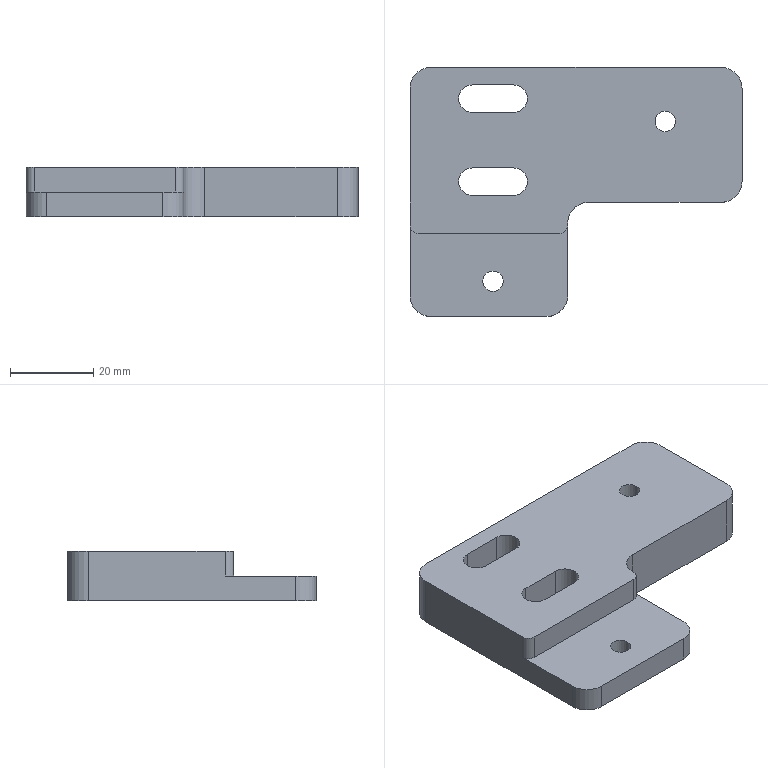NC program | NX | posted with a generic post | part box 80 x 60 x 12 mm
Lines 19 to 945 of 5338:
(ADAPTIVE_MILLING , TOOL : D10)
N36 T15 M6
N38 G54
N40 G17 G0 G90 X-52.678 Y3.969 S9500 M3
N42 G43 Z30. H15
N44 Z-9.
N46 G94 G1 Z-12. F1000.
N48 X-51.955 Y3.649 F3500.
N50 X-51.222 Y3.352
N52 G3 X-50.031 Y3.969 R1.015
N54 X-49.59 Y7.203 R11.435
N56 X-49.506 Y16.827 R445.113
N58 G2 X-49.477 Y33.326 R953.284
N60 X-46.244 Y37.824 R6.109
N62 X-40.67 Y39.298 R13.456
N64 X-30.424 Y39.492 R151.23
N66 G1 X-24.674 Y39.494
N68 X42.826
N70 X42.951 Y39.492
N72 X43.076 Y39.487
N74 X43.138 Y39.483
N76 X43.263 Y39.472
N78 G2 X47.822 Y36.232 R6.088
N80 X49.287 Y30.783 R13.246
N82 X49.492 Y20.413 R143.675
N84 G1 X49.494 Y14.85
N86 Y-32.837
N88 X49.492 Y-32.962
N90 X49.487 Y-33.087
N92 X49.483 Y-33.15
N94 X49.472 Y-33.274
N96 G2 X46.278 Y-37.797 R6.078
N98 X40.71 Y-39.294 R13.263
N100 X31.027 Y-39.491 R137.718
N102 G1 X26.59 Y-39.493
N104 X-35.848 Y-39.494
N106 X-36.098 Y-39.495
N108 X-42.848
N110 X-42.973 Y-39.492
N112 X-43.098 Y-39.487
N114 G2 X-47.739 Y-36.377 R5.989
N116 X-49.266 Y-31.012 R12.765
N118 X-49.491 Y-21.58 R116.088
N120 G1 X-49.494 Y-17.955
N122 Y1.295
N124 X-49.491 Y1.545
N126 X-49.483 Y1.795
N128 X-49.473 Y2.045
N130 G3 X-49.015 Y15.406 R138.865
N132 G2 X-48.982 Y31.281 R941.095
N134 X-44.875 Y37.18 R7.48
N136 X-38.995 Y38.738 R15.237
N138 X-29.501 Y38.983 R119.88
N140 G1 X-26.813 Y38.987
N142 X-20.001 Y38.988
N144 X40.687
N146 X40.812 Y38.986
N148 X40.937 Y38.983
N150 X41.124 Y38.973
N152 G2 X47.135 Y34.939 R7.429
N154 X48.754 Y28.822 R15.356
N156 X48.985 Y18.827 R132.025
N158 G1 X48.988 Y15.452
N160 X48.989 Y-0.298
N162 Y-30.673
N164 X48.987 Y-30.798
N166 X48.981 Y-30.985
N168 X48.975 Y-31.11
N170 G2 X44.898 Y-37.158 R7.437
N172 X38.899 Y-38.747 R15.354
N174 X28.53 Y-38.985 R135.396
N176 G1 X24.842 Y-38.988
N178 X-3.845
N180 X-33.72 Y-38.989
N182 X-35.845
N184 X-40.658
N186 X-40.783 Y-38.988
N188 G2 X-47.121 Y-34.966 R7.396
N190 X-48.734 Y-29.039 R15.01
N192 X-48.982 Y-20.17 R108.447
N194 G1 X-48.986 Y-17.92
N196 X-48.988 Y-13.482
N198 Y-0.42
N200 X-48.985 Y0.08
N202 X-48.979 Y0.392
N204 X-48.968 Y0.83
N206 G3 X-48.519 Y18.07 R239.849
N208 G2 X-48.482 Y29.632 R716.485
N210 X-43.532 Y36.705 R8.46
N212 X-37.316 Y38.227 R17.447
N214 X-27.509 Y38.477 R128.145
N216 G1 X-24.822 Y38.481
N218 X-18.884 Y38.483
N220 X23.928
N222 X24.241 Y38.484
N224 X24.803
N226 X25.116 Y38.485
N228 G2 X39.678 Y38.452 R836.944
N230 X46.698 Y33.525 R8.442
N232 X48.256 Y26.999 R17.862
N234 X48.481 Y15.129 R177.604
N236 G1 X48.483 Y9.879
N238 Y-28.746
N240 X48.481 Y-28.996
N242 X48.477 Y-29.184
N244 X48.473 Y-29.309
N246 X48.464 Y-29.496
N248 G2 X43.52 Y-36.701 R8.44
N250 X36.993 Y-38.255 R17.932
N252 X26.123 Y-38.479 R161.092
N254 G1 X22.373 Y-38.482
N256 X-1.002 Y-38.483
N258 X-23.377
N260 X-23.689 Y-38.484
N262 X-24.252
N264 X-24.564 Y-38.485
N266 G2 X-39.689 Y-38.454 R869.538
N268 X-46.704 Y-33.517 R8.449
N270 X-48.245 Y-27.115 R17.733
N272 X-48.48 Y-15.995 R158.486
N274 X-48.427 Y1.004 R748.676
N276 G3 X-48.025 Y18.685 R293.67
N278 G2 X-47.965 Y28.433 R262.553
N280 X-42.389 Y36.207 R9.207
N282 X-35.598 Y37.743 R19.721
N284 X-23.165 Y37.975 R191.105
N286 G1 X-18.165 Y37.977
N288 X21.835 Y37.978
N290 X22.273 Y37.979
N292 X22.71 Y37.98
N294 X23.148 Y37.981
N296 X24.585 Y37.98
N298 G2 X38.334 Y37.943 R554.072
N300 X46.194 Y32.397 R9.198
N302 X47.727 Y25.797 R19.223
N304 X47.973 Y15.115 R152.13
N306 G1 X47.976 Y12.177
N308 X47.978 Y4.927
N310 Y-27.073
N312 X47.976 Y-27.385
N314 X47.971 Y-27.635
N316 X47.968 Y-27.76
N318 G2 X42.406 Y-36.188 R9.21
N320 X35.557 Y-37.743 R19.566
N322 X23.749 Y-37.974 R179.522
N324 G1 X19.437 Y-37.977
N326 X-21.251 Y-37.978
N328 X-22.376 Y-37.979
N330 X-22.813 Y-37.98
N332 X-24.626
N334 X-26.063 Y-37.981
N336 G2 X-38.313 Y-37.944 R530.442
N338 X-46.185 Y-32.418 R9.187
N340 X-47.724 Y-25.819 R19.251
N342 X-47.974 Y-14.324 R163.209
N344 X-47.899 Y1.05 R522.369
N346 G3 X-47.526 Y22.169 R410.142
N348 G2 X-47.395 Y27.851 R55.442
N350 X-41.366 Y35.698 R9.806
N352 X-34.567 Y37.213 R20.757
N354 X-23.635 Y37.466 R154.256
N356 G1 X-20.76 Y37.47
N358 X-14.385 Y37.472
N360 X19.553
N362 X20.115 Y37.474
N364 X20.678
N366 X21.178 Y37.476
N368 G2 X36.865 Y37.45 R878.1
N370 X45.705 Y31.332 R9.835
N372 X47.23 Y24.345 R21.115
N374 X47.469 Y11.912 R192.215
N376 G1 X47.472 Y7.474
N378 Y-25.588
N380 X47.47 Y-25.901
N382 X47.464 Y-26.275
N384 X47.457 Y-26.525
N386 X47.447 Y-26.775
N388 G2 X41.351 Y-35.693 R9.827
N390 X34.366 Y-37.227 R21.025
N392 X22.058 Y-37.469 R187.16
N394 G1 X17.621 Y-37.472
N396 X-19.067
N398 X-19.567 Y-37.474
N400 X-20.379
N402 X-21.067 Y-37.475
N404 X-22.442
N406 G2 X-36.941 Y-37.445 R794.612
N408 X-45.735 Y-31.262 R9.832
N410 X-47.246 Y-24.144 R21.676
N412 X-47.468 Y-12.961 R184.381
N414 X-47.154 Y7.847 R395.574
N416 G3 X-47.008 Y25.033 R897.934
N418 G2 X-45.105 Y31.525 R11.201
N420 X-38.676 Y35.814 R11.777
N422 X-31.077 Y36.842 R31.833
N424 X-12.078 Y36.967 R673.573
N426 G1 X17.422
N428 X19.922 Y36.97
N430 X21.422 Y36.971
N432 X21.859 Y36.973
N434 X22.546 Y36.974
N436 X23.359
N438 G2 X35.796 Y36.94 R601.467
N440 X45.211 Y30.341 R10.368
N442 X46.723 Y23.157 R22.585
N444 X46.964 Y10.099 R209.815
N446 G1 X46.967 Y5.287
N448 Y-24.213
N450 X46.963 Y-24.713
N452 X46.958 Y-25.026
N454 X46.95 Y-25.338
N456 G2 X44.37 Y-32.399 R10.607
N458 X37.985 Y-35.996 R12.565
N460 X30.049 Y-36.876 R37.4
N462 X13.987 Y-36.966 R769.024
N464 G1 X-16.888 Y-36.967
N466 X-17.325 Y-36.968
N468 X-18.263 Y-36.969
N470 X-19.513 Y-36.97
N472 X-20.263
N474 X-20.763 Y-36.971
N476 G2 X-35.824 Y-36.936 R721.83
N478 X-45.174 Y-30.43 R10.334
N480 X-46.712 Y-23.316 R22.255
N482 X-46.963 Y-11.383 R181.717
N484 X-46.662 Y7.862 R420.02
N486 G3 X-46.505 Y24.049 R969.988
N488 G2 X-44.748 Y30.472 R12.025
N490 X-38.349 Y35.114 R11.8
N492 X-30.526 Y36.307 R29.809
N494 X-13.59 Y36.461 R466.972
N496 G1 X15.223 Y36.462
N498 X16.035
N500 X16.473 Y36.464
N502 X16.91
N504 X17.223 Y36.465
N506 X18.535
N508 G2 X34.597 Y36.44 R831.129
N510 X41.935 Y33.566 R11.003
N512 X45.507 Y26.949 R13.263
N514 X46.376 Y18.635 R40.48
N516 X46.462 Y0.51 R850.421
N518 G1 Y-22.865
N520 X46.458 Y-23.427
N522 X46.453 Y-23.74
N524 X46.444 Y-24.114
N526 X46.436 Y-24.364
N528 G2 X44.121 Y-31.289 R11.301
N530 X37.648 Y-35.319 R12.461
N532 X29.858 Y-36.334 R33.754
N534 X12.296 Y-36.461 R612.464
N536 G1 X-14.704 Y-36.462
N538 X-15.141 Y-36.463
N540 X-16.141 Y-36.464
N542 X-16.641 Y-36.465
N544 X-18.078
N546 X-18.516 Y-36.466
N548 G2 X-34.765 Y-36.428 R731.931
N550 X-44.669 Y-29.518 R10.799
N552 X-46.194 Y-22.335 R23.117
N554 X-46.457 Y-10.153 R180.72
N556 X-46.151 Y8.531 R482.227
N558 G3 X-46.014 Y22.718 R881.104
N560 G2 X-44.715 Y28.837 R13.812
N562 X-42.3 Y31.949 R10.683
N564 X-38.4 Y34.48 R10.149
N566 X-31.457 Y35.691 R27.998
N568 X-19.337 Y35.95 R192.668
N570 G1 X-16.275 Y35.954
N572 X-10.087 Y35.956
N574 X13.038
N576 X13.913 Y35.957
N578 X14.35 Y35.959
N580 X14.913
N582 X15.788 Y35.96
N584 X16.1 Y35.961
N586 X16.6
N588 X16.913 Y35.963
N590 X17.475
N592 X17.85 Y35.964
N594 X18.163
N596 X18.538 Y35.966
N598 X19.038
N600 X19.975 Y35.97
N602 X20.538 Y35.969
N604 X21.913 Y35.973
N606 X22.85 Y35.976
N608 X23.35
N610 X23.725 Y35.977
N612 X25.288 Y35.975
N614 X26.163 Y35.978
N616 X26.663 Y35.977
N618 X27.288 Y35.979
N620 X27.663
N622 X28.413 Y35.981
N624 X28.913 Y35.98
N626 X29.35 Y35.981
N628 G2 X35.217 Y35.785 R46.802
N630 X41.859 Y32.374 R10.751
N632 G1 X42.103 Y32.174
N634 X42.174 Y32.103
N636 X43.366 Y30.65
N638 X43.422 Y30.567
N640 G2 X44.442 Y28.519 R12.875
N642 X45.67 Y21.706 R27.357
N644 X45.952 Y8.337 R197.475
N646 G1 X45.955 Y4.587
N648 X45.956 Y-6.163
N650 Y-21.663
N652 X45.952 Y-22.226
N654 X45.945 Y-22.726
N656 X45.936 Y-23.101
N658 G2 X44.27 Y-29.558 R12.646
N660 X37.727 Y-34.507 R11.976
N662 X30.041 Y-35.766 R28.902
N664 X14.044 Y-35.955 R359.108
N666 G1 X-0.956 Y-35.956
N668 X-12.519
N670 X-13.019 Y-35.958
N672 X-14.019 Y-35.959
N674 X-14.456 Y-35.96
N676 X-15.644
N678 G2 X-33.643 Y-35.926 R895.197
N680 X-40.761 Y-33.419 R11.64
N682 X-43.422 Y-30.567 R16.586
N684 X-44.442 Y-28.519 R12.875
N686 X-45.681 Y-21.581 R27.69
N688 X-45.949 Y-9.837 R179.438
N690 X-45.644 Y9.347 R619.345
N692 G1 X-45.614 Y11.034
N694 X-45.597 Y12.097
N696 X-45.584 Y13.534
N698 X-45.572 Y15.221
N700 X-45.566 Y16.409
N702 X-45.563 Y16.846
N704 X-45.561 Y17.346
N706 X-45.558 Y17.784
N708 X-45.556 Y18.159
N710 X-45.548 Y19.159
N712 X-45.547 Y19.471
N714 X-45.537 Y20.409
N716 X-45.526 Y21.221
N718 X-45.516 Y21.659
N720 X-45.503 Y22.096
N722 X-45.49 Y22.408
N724 G2 X-45.012 Y25.891 R17.523
N726 G1 X-44.911 Y26.92
N728 X-44.891 Y27.019
N730 X-44.346 Y28.817
N732 X-44.307 Y28.91
N734 X-43.422 Y30.567
N736 X-43.366 Y30.65
N738 X-42.295 Y31.955
N740 X-42.103 Y32.174
N742 X-41.341 Y32.806
N744 X-40.567 Y33.422
N746 X-39.697 Y33.893
N748 X-38.817 Y34.346
N750 X-37.019 Y34.891
N752 G2 X-32.663 Y35.155 R39.026
N754 X-16.23 Y35.447 R314.936
N756 G1 X-11.418 Y35.45
N758 X10.895 Y35.451
N760 X11.77 Y35.452
N762 X12.27 Y35.454
N764 X12.832
N766 X13.707 Y35.455
N768 X14.145 Y35.457
N770 X14.707
N772 X15.457 Y35.458
N774 X15.895 Y35.46
N776 X16.332
N778 X17.082 Y35.461
N780 X18.27 Y35.464
N782 X18.582
N784 X19.02 Y35.466
N786 X20.395 Y35.468
N788 X21.332 Y35.47
N790 X22.207 Y35.471
N792 X23.207
N794 X23.707 Y35.472
N796 X24.332 Y35.473
N798 X24.582
N800 X25.02 Y35.474
N802 X26.02 Y35.475
N804 X27.707 Y35.476
N806 G2 X34.138 Y35.299 R59.033
N808 G3 X37.019 Y34.891 R34.04
N810 G1 X38.817 Y34.346
N812 X38.91 Y34.307
N814 X40.567 Y33.422
N816 X40.65 Y33.366
N818 X41.907 Y32.335
N820 G3 X43.412 Y32.617 R1.003
N822 X43.466 Y33.5 Z-11.954 R1.05
N824 G1 X43.142 Y34.537 Z-11.9
N826 X42.635 Y36.159
N828 G3 X41.907 Y36.835 R1.014
N830 G1 X38.497 Y37.613
N832 G3 X30.566 Y38.446 R43.677
N834 G1 X29.568 Y38.454
N836 X-29.332 Y38.314
N838 X-30.98 Y38.282
N840 X-31.144 Y38.26
N842 X-31.304 Y38.22
N844 X-32.966 Y37.607
N846 X-34.617 Y36.991 Z-11.988
N848 X-34.814 Y36.858 Z-12.
N850 G3 X-34.162 Y35.1 R1.001
N852 G1 X34.975
N854 X35.025 Y35.098
N856 X35.647 Y35.036
N858 X36.334 Y34.972
N860 X37.019 Y34.891
N862 X37.968 Y34.61
N864 X38.91 Y34.307
N866 X39.785 Y33.846
N868 X40.65 Y33.366
N870 X41.419 Y32.742
N872 X42.174 Y32.103
N874 X42.806 Y31.341
N876 X43.422 Y30.567
N878 X43.893 Y29.697
N880 X44.346 Y28.817
N882 X44.891 Y27.019
N884 G2 X45.137 Y23.038 R31.355
N886 X45.449 Y4.73 R341.606
N888 G1 X45.451 Y-2.707
N890 Y-20.52
N892 X45.446 Y-21.145
N894 X45.441 Y-21.582
N896 X45.431 Y-22.019
N898 G2 X44.027 Y-28.303 R13.841
N900 X37.349 Y-33.834 R11.954
N902 X29.375 Y-35.239 R28.194
N904 X15.816 Y-35.448 R271.557
N906 G1 X10.754 Y-35.45
N908 X-10.246 Y-35.451
N910 X-10.809 Y-35.453
N912 X-11.871
N914 X-12.309 Y-35.455
N916 X-13.559
N918 X-13.996 Y-35.457
N920 X-14.621
N922 X-15.059 Y-35.459
N924 X-15.434
N926 X-15.809 Y-35.461
N928 X-18.121 Y-35.462
N930 X-18.434 Y-35.464
N932 X-19.246
N934 X-19.809 Y-35.466
N936 X-20.559
N938 X-20.996 Y-35.467
N940 X-21.434
N942 X-21.996 Y-35.469
N944 X-24.246 Y-35.468
N946 X-25.121 Y-35.469
N948 X-25.559 Y-35.47
N950 X-27.559
N952 G2 X-34.115 Y-35.298 R62.042
N954 G3 X-37.019 Y-34.891 R35.555
N956 G1 X-38.817 Y-34.346
N958 X-38.91 Y-34.307
N960 X-40.567 Y-33.422
N962 X-40.65 Y-33.366
N964 X-41.858 Y-32.374
N966 G3 X-43.408 Y-32.714 R1.013
N968 G1 X-43.716 Y-33.336
N970 X-43.999 Y-33.968
N972 G3 X-42.476 Y-35.092 R1.011
N974 G1 Z-9.
N976 G0 Z53.
N978 X47.598 Y23.655
N980 Z-9.
N982 G1 Z-12. F1000.
N984 G3 X46.702 Y25.451 R1.01 F3500.
N986 G1 X46.161 Y25.257
N988 X45.625 Y25.048
N990 G3 X45.1 Y24.162 R1.021
N992 G1 Y2.525
N994 X45.098 Y2.475
N996 X45.085 Y2.288
N998 G3 X44.958 Y-7.648 R217.132
N1000 G2 X44.896 Y-21.834 R589.05
N1002 X42.728 Y-28.839 R12.853
N1004 X35.905 Y-33.542 R12.934
N1006 X27.644 Y-34.774 R32.85
N1008 X11.897 Y-34.944 R414.031
N1010 G1 X1.147 Y-34.945
N1012 X-5.416
N1014 X-5.435 Y-34.946
N1016 X-6.975 Y-35.098
N1018 X-7.025 Y-35.1
N1020 X-34.975
N1022 X-35.025 Y-35.098
N1024 X-35.647 Y-35.036
N1026 G3 X-36.243 Y-36.899 R1.
N1028 G1 X-35.582 Y-37.161 Z-11.964
N1030 X-34.911 Y-37.397 Z-11.929
N1032 X-34.369 Y-37.593 Z-11.9
N1034 X-32.805 Y-38.159
N1036 X-32.637 Y-38.199
N1038 X-32.465 Y-38.218
N1040 X23.16
N1042 G3 X31.85 Y-37.499 R53.484
N1044 G1 X33.699 Y-37.193
N1046 X35.545 Y-36.87
N1048 G3 X39.608 Y-35.33 R13.765
N1050 G1 X41.159 Y-34.433
N1052 X42.699 Y-33.516
N1054 G3 X44.937 Y-31.231 R7.798
N1056 X47.702 Y-23.575 R18.416
N1058 X47.923 Y-20.596 R27.932
N1060 G1 X48.28 Y-0.707
N1062 X48.26 Y-0.515
N1064 X48.212 Y-0.328
N1066 X47.523 Y1.451
N1068 X47.251 Y2.168 Z-11.938
N1070 X46.958 Y2.878 Z-11.977
N1072 X46.817 Y3.061 Z-11.988
N1074 X46.642 Y3.213 Z-12.
N1076 G3 X45.098 Y2.475 R1.002
N1078 G2 X44.671 Y-0.875 R42.456
N1080 G3 X44.468 Y-8.307 R92.385
N1082 G2 X44.375 Y-21.243 R367.805
N1084 X42.069 Y-28.332 R13.004
N1086 X34.975 Y-33.075 R13.335
N1088 X26.707 Y-34.267 R34.294
N1090 X11.896 Y-34.438 R394.662
N1092 G1 X4.709 Y-34.44
N1094 X-3.291
N1096 X-3.354
N1098 X-3.416 Y-34.443
N1100 X-3.479 Y-34.449
N1102 X-3.54 Y-34.459
N1104 X-3.561 Y-34.46
N1106 G2 X-5.453 Y-34.948 R8.588
N1108 G3 X-6.25 Y-36.389 R1.002
N1110 X-5.534 Y-36.946 Z-11.953 R1.152
N1112 G1 X-4.54 Y-37.328 Z-11.9
N1114 X-2.514 Y-38.1
N1116 X-2.271 Y-38.13
N1118 X16.479
N1120 G3 X28.916 Y-37.246 R88.684
N1122 G1 X33.862 Y-36.528
N1124 G3 X38.571 Y-34.974 R16.748
N1126 G1 X39.382 Y-34.514
N1128 X40.164 Y-34.007
N1130 X42.71 Y-32.209
N1132 G3 X43.858 Y-31.165 R6.533
N1134 G1 X44.638 Y-30.074
N1136 X45.399 Y-28.969
N1138 G3 X46.659 Y-26.003 R10.818
N1140 G1 X46.864 Y-25.092
N1142 X47.023 Y-24.172
N1144 G3 X47.4 Y-20.454 R30.837
N1146 G1 X48.073 Y-2.701
N1148 X48.053 Y-2.481
N1150 X47.993 Y-2.268
N1152 X47.227 Y-0.485
N1154 X46.969 Y0.129 Z-11.933
N1156 X46.689 Y0.733 Z-11.967
N1158 G3 X46.172 Y1.137 Z-12. R1.04
N1160 X44.891 Y0.481 R1.004
N1162 X44.059 Y-4.805 R16.614
N1164 X43.927 Y-19.054 R945.857
N1166 G2 X42.801 Y-25.414 R17.122
N1168 X35.689 Y-32.053 R12.395
N1170 X27.565 Y-33.657 R27.487
N1172 X14.946 Y-33.927 R202.133
N1174 G1 X11.946 Y-33.931
N1176 X6.571 Y-33.934
N1178 X-1.117 Y-33.935
N1180 X-1.617 Y-33.938
N1182 X-1.867 Y-33.942
N1184 X-2.054 Y-33.948
N1186 G3 X-3.183 Y-34.346 R2.382
N1188 G1 X-3.602 Y-34.473
N1190 G3 X-4.272 Y-35.709 R1.005
N1192 X-3.531 Y-36.423 Z-11.946 R1.111
N1194 G1 X-2.677 Y-36.785 Z-11.9
N1196 X-0.684 Y-37.619
N1198 X-0.42 Y-37.655
N1200 X16.455
N1202 G3 X27.648 Y-36.859 R79.831
N1204 G1 X31.563 Y-36.288
N1206 G3 X36.264 Y-35.046 R28.073
N1208 X40.025 Y-33.091 R17.846
N1210 G1 X42.078 Y-31.672
N1212 G3 X43.232 Y-30.634 R6.485
N1214 G1 X44.018 Y-29.548
N1216 X44.786 Y-28.448
N1218 G3 X46.067 Y-25.491 R10.891
N1220 G1 X46.281 Y-24.581
N1222 X46.448 Y-23.663
N1224 G3 X46.87 Y-19.949 R32.118
N1226 G1 X47.71 Y-3.897
N1228 X47.692 Y-3.669
N1230 X47.63 Y-3.448
N1232 X46.866 Y-1.679
N1234 X46.606 Y-1.066 Z-11.933
N1236 X46.325 Y-0.462 Z-11.967
N1238 G3 X45.808 Y-0.059 Z-12. R1.04
N1240 X44.528 Y-0.715 R1.004
N1242 X43.846 Y-3.157 R15.616
N1244 X43.496 Y-10.143 R54.908
N1246 G2 X43.331 Y-20.077 R185.707
N1248 X40.455 Y-27.728 R13.17
N1250 X33.132 Y-32.149 R14.342
N1252 X24.412 Y-33.278 R38.601
N1254 X8.851 Y-33.427 R508.578
N1256 G3 X-1.335 Y-33.484 R275.552
N1258 X-2.618 Y-34.055 R3.84
N1260 X-3.12 Y-35.165 R1.007
N1262 X-2.413 Y-35.918 Z-11.946 R1.108
N1264 G1 X-1.581 Y-36.317 Z-11.9
N1266 X-0.66 Y-36.765
N1268 X0.27 Y-37.193
N1270 X0.564 Y-37.237
N1272 X13.689
N1274 G3 X27.37 Y-36.265 R97.54
N1276 G1 X30.153 Y-35.872
N1278 X32.933 Y-35.457
N1280 G3 X37.927 Y-33.604 R16.39
N1282 G1 X38.569 Y-33.221
N1284 X39.199 Y-32.819
N1286 X40.969 Y-31.609
N1288 G3 X42.397 Y-30.245 R9.113
N1290 X44.176 Y-27.844 R25.524
N1292 X45.244 Y-25.469 R11.428
N1294 X46.166 Y-21.226 R17.742
N1296 G1 X46.426 Y-18.742
N1298 X46.639 Y-16.254
N1300 X47.489 Y-4.592
N1302 G3 X47.389 Y-4.076 R1.064
N1304 G1 X46.591 Y-2.462
N1306 X46.305 Y-1.871 Z-11.933
N1308 X45.997 Y-1.292 Z-11.966
N1310 G3 X45.44 Y-0.913 Z-12. R1.039
N1312 X44.307 Y-1.41 R1.007
N1314 X43.273 Y-5.045 R8.478
N1316 X42.975 Y-14.6 R110.984
N1318 G2 X42.583 Y-21.205 R41.356
N1320 X34.846 Y-30.789 R12.558
N1322 X26.889 Y-32.566 R25.976
N1324 X15.335 Y-32.908 R150.656
N1326 G3 X-0.164 Y-32.976 R823.63
N1328 X-1.433 Y-33.422 R1.799
N1330 G1 X-1.764 Y-33.598
N1332 G3 X-2.268 Y-34.703 R1.007
N1334 X-1.56 Y-35.461 Z-11.946 R1.106
N1336 G1 X-0.733 Y-35.858 Z-11.9
N1338 X0.191 Y-36.307
N1340 X1.124 Y-36.736
N1342 X1.418 Y-36.78
N1344 X6.104 Y-36.786
N1346 X10.791 Y-36.768
N1348 G3 X23.872 Y-35.952 R137.075
N1350 G1 X29.666 Y-35.297
N1352 G3 X35.088 Y-34.021 R28.468
N1354 X39.35 Y-31.863 R18.807
N1356 X42.089 Y-29.371 R14.73
N1358 G1 X43.211 Y-28.032
N1360 G3 X45.058 Y-23.989 R10.649
N1362 X45.72 Y-19.688 R23.394
N1364 X46.263 Y-5.858 R425.517
N1366 G1 X46.149 Y-4.697
N1368 X46.02 Y-3.537
N1370 X45.95 Y-2.853 Z-11.934
N1372 X45.86 Y-2.171 Z-11.969
N1374 G3 X45.525 Y-1.656 Z-12. R1.045
N1376 X44.013 Y-1.961 R1.003
N1378 X42.805 Y-5.996 R9.156
N1380 X42.48 Y-14.549 R100.058
N1382 G2 X41.984 Y-20.957 R34.687
N1384 X34.161 Y-30.277 R12.756
N1386 X26.077 Y-32.06 R26.564
N1388 X14.148 Y-32.403 R157.798
N1390 G3 X0.774 Y-32.481 R593.839
N1392 X-0.638 Y-32.781 R3.263
N1394 G1 X-1.169 Y-33.218
N1396 G3 X-1.398 Y-34.494 R1.006
N1398 X-0.497 Y-35.007 Z-11.946 R1.107
N1400 G1 X0.411 Y-35.139 Z-11.9
N1402 X1.568 Y-35.314
N1404 X2.728 Y-35.468
N1406 X20.228
N1408 G3 X28.933 Y-34.795 R59.876
N1410 X35.524 Y-32.99 R26.706
N1412 X38.471 Y-31.272 R16.801
N1414 X41.07 Y-29.185 R27.273
N1416 X43.338 Y-26.004 R11.083
N1418 X45.224 Y-18.962 R18.255
N1420 G1 X45.407 Y-16.472
N1422 X45.537 Y-13.979
N1424 X45.821 Y-6.685
N1426 X45.71 Y-5.513
N1428 X45.577 Y-4.344
N1430 X45.507 Y-3.668 Z-11.934
N1432 X45.417 Y-2.994 Z-11.968
N1434 G3 X45.068 Y-2.471 Z-12. R1.043
N1436 X43.571 Y-2.788 R1.004
N1438 X42.393 Y-6.419 R8.205
N1440 X41.995 Y-14.092 R75.737
N1442 G2 X41.414 Y-20.555 R32.895
N1444 X33.512 Y-29.754 R12.939
N1446 X25.428 Y-31.54 R26.713
N1448 X13.062 Y-31.898 R158.607
N1450 G3 X1.438 Y-32. R310.835
N1452 X-0.109 Y-32.348 R3.396
N1454 G1 X-0.641 Y-32.784
N1456 G3 X-0.873 Y-34.057 R1.006
N1458 X-0.052 Y-34.561 Z-11.95 R1.037
N1460 G1 X0.935 Y-34.705 Z-11.9
N1462 X2.094 Y-34.881
N1464 X3.256 Y-35.034
N1466 X20.756
N1468 G3 X28.196 Y-34.363 R42.087
N1470 G1 X30.774 Y-33.882
N1472 G3 X35.926 Y-32.053 R20.327
N1474 X38.51 Y-30.479 R36.816
N1476 X41.267 Y-27.866 R13.081
N1478 X43.202 Y-24.683 R12.875
N1480 X44.351 Y-21.133 R20.534
N1482 G1 X44.51 Y-20.214
N1484 X44.618 Y-19.288
N1486 X45.618 Y-6.932
N1488 X45.296 Y-4.752
N1490 X45.204 Y-4.107 Z-11.933
N1492 X45.087 Y-3.466 Z-11.965
N1494 G3 X44.661 Y-2.932 Z-12. R1.038
N1496 X43.366 Y-3.15 R1.005
N1498 X42.157 Y-5.856 R5.599
N1500 X41.576 Y-12.008 R36.865
N1502 G2 X41.091 Y-18.986 R53.966
N1504 X32.934 Y-29.208 R13.156
N1506 X24.606 Y-31.039 R27.296
N1508 X10.926 Y-31.397 R182.226
N1510 G3 X1.929 Y-31.53 R155.418
N1512 X0.367 Y-31.914 R3.46
N1514 G1 X0.318 Y-31.953
N1516 X0.271 Y-31.994
N1518 X0.248 Y-32.012
N1520 X0.174 Y-32.103
N1522 X0.103 Y-32.174
N1524 X-0.139 Y-32.372
N1526 G3 X-0.373 Y-33.641 R1.006
N1528 X0.449 Y-34.149 Z-11.95 R1.037
N1530 G1 X1.433 Y-34.293 Z-11.9
N1532 X2.594 Y-34.469
N1534 X3.758 Y-34.622
N1536 X19.383
N1538 G3 X28.048 Y-33.764 R44.556
N1540 G1 X31.108 Y-33.14
N1542 G3 X37.268 Y-30.26 R17.21
N1544 X40.063 Y-27.966 R25.973
N1546 X42.572 Y-24.286 R11.548
N1548 X44.001 Y-19.537 R18.76
N1550 X44.683 Y-14.597 R55.586
N1552 G1 X45.342 Y-7.265
N1554 X45.02 Y-5.092
N1556 X44.927 Y-4.446 Z-11.933
N1558 X44.809 Y-3.804 Z-11.965
N1560 G3 X44.385 Y-3.271 Z-12. R1.038
N1562 X43.088 Y-3.489 R1.005
N1564 X41.695 Y-6.515 R6.092
N1566 X41.06 Y-13.101 R41.667
N1568 G2 X40.33 Y-19.549 R32.749
N1570 X32.198 Y-28.732 R13.317
N1572 X23.987 Y-30.52 R27.65
N1574 X10.308 Y-30.894 R181.55
N1576 G3 X2.437 Y-31.056 R109.458
N1578 X0.65 Y-31.551 R3.758
N1580 G1 X0.603 Y-31.592
N1582 X0.577 Y-31.612
N1584 X0.22 Y-32.047
N1586 G3 X0.114 Y-33.158 R1.01
N1588 X0.983 Y-33.698 Z-11.947 R1.113
N1590 G1 X1.899 Y-33.879 Z-11.9
N1592 X4.02 Y-34.292
N1594 X15.992 Y-34.297
N1596 G3 X24.691 Y-33.631 R57.899
N1598 G1 X26.604 Y-33.336
N1600 X28.507 Y-32.983
N1602 G3 X32.742 Y-31.744 R28.951
N1604 X35.904 Y-30.15 R20.132
N1606 G1 X38.014 Y-28.82
N1608 G3 X39.218 Y-27.837 R7.261
N1610 G1 X40.082 Y-26.81
N1612 X40.932 Y-25.772
N1614 G3 X42.831 Y-21.75 R10.863
N1616 X44.004 Y-15.629 R52.6
N1618 G1 X44.981 Y-7.821
N1620 X44.977 Y-7.544
N1622 X44.666 Y-5.528
N1624 X44.571 Y-4.881 Z-11.933
N1626 X44.452 Y-4.238 Z-11.966
N1628 G3 X44.03 Y-3.707 Z-12. R1.038
N1630 X42.731 Y-3.923 R1.005
N1632 X41.266 Y-6.985 R6.238
N1634 X40.588 Y-13.002 R38.872
N1636 G2 X39.726 Y-19.306 R30.222
N1638 X31.651 Y-28.181 R13.481
N1640 X23.259 Y-30.013 R28.046
N1642 X10.267 Y-30.387 R176.141
N1644 G3 X2.836 Y-30.593 R82.988
N1646 X0.995 Y-31.129 R4.054
N1648 G1 X0.948 Y-31.17
N1650 X0.903 Y-31.214
N1652 X0.546 Y-31.649
N1654 G3 X0.454 Y-32.785 R1.01
N1656 X1.22 Y-33.283 Z-11.953 R1.046
N1658 G1 X2.254 Y-33.487 Z-11.9
N1660 X4.346 Y-33.894
N1662 X9.784 Y-33.905
N1664 X15.221 Y-33.884
N1666 G3 X24.992 Y-32.974 R68.769
N1668 G1 X28.362 Y-32.397
N1670 G3 X34.473 Y-30.356 R27.25
N1672 X37.979 Y-27.863 R13.069
N1674 G1 X38.774 Y-27.07
N1676 X39.538 Y-26.247
N1678 G3 X41.623 Y-22.862 R14.267
N1680 X42.924 Y-18.723 R15.383
N1682 G1 X44.545 Y-8.352
N1684 Y-8.042
N1686 X44.233 Y-6.06
N1688 X44.137 Y-5.412 Z-11.933
N1690 X44.015 Y-4.767 Z-11.966
N1692 G3 X43.595 Y-4.239 Z-12. R1.038
N1694 X42.295 Y-4.455 R1.005
N1696 X40.884 Y-7.243 R5.706
N1698 X40.118 Y-12.935 R35.302
N1700 G2 X39.011 Y-19.385 R26.693
N1702 X30.853 Y-27.738 R13.726
N1704 X22.384 Y-29.52 R29.026
N1706 X9.955 Y-29.882 R175.848
N1708 G3 X3.151 Y-30.138 R62.165
N1710 X1.324 Y-30.715 R3.841
N1712 G1 X1.279 Y-30.758
N1714 X1.264 Y-30.775
N1716 X0.867 Y-31.258
N1718 G3 X0.774 Y-32.392 R1.01
N1720 X1.541 Y-32.892 Z-11.953 R1.045
N1722 G1 X2.572 Y-33.095 Z-11.9
N1724 X4.667 Y-33.503
N1726 X8.331 Y-33.509
N1728 X11.994 Y-33.493
N1730 G3 X21.59 Y-32.764 R86.058
N1732 G1 X24.439 Y-32.389
N1734 X27.286 Y-31.992
N1736 G3 X34.418 Y-29.325 R19.872
N1738 X37.24 Y-27.386 R28.048
N1740 X41.545 Y-21.265 R14.049
N1742 X42.362 Y-18.397 R19.989
N1744 G1 X44.353 Y-8.571
N1746 X44.369 Y-8.365
N1748 X44.35 Y-8.16
N1750 X43.96 Y-6.366
N1752 X43.824 Y-5.717 Z-11.933
N1754 X43.665 Y-5.074 Z-11.966
N1756 G3 X43.229 Y-4.576 Z-12. R1.04
N1758 X42.103 Y-4.674 R1.01
N1760 X40.661 Y-6.963 R4.46
N1762 X39.664 Y-12.741 R27.927
N1764 G2 X38.383 Y-19.158 R25.785
N1766 X30.299 Y-27.199 R13.922
N1768 X21.584 Y-29.021 R29.569
N1770 X9.092 Y-29.388 R192.514
N1772 G3 X3.233 Y-29.722 R40.566
N1774 X1.609 Y-30.317 R3.393
N1776 G1 X1.566 Y-30.362
N1778 X1.525 Y-30.41
N1780 X1.487 Y-30.459
N1782 X1.452 Y-30.511
N1784 G3 X1.472 Y-31.491 R1.014
N1786 X2.265 Y-31.997 Z-11.952 R1.132
N1788 G1 X3.26 Y-32.254 Z-11.9
N1790 X5.223 Y-32.753
N1792 X9.972 Y-32.764
N1794 X14.722 Y-32.748
N1796 G3 X23.417 Y-31.965 R66.337
N1798 X30.717 Y-30.321 R50.646
N1800 X35.466 Y-27.978 R14.488
N1802 X37.036 Y-26.547 R13.092
N1804 G1 X37.883 Y-25.631
N1806 X38.692 Y-24.681
N1808 G3 X41.47 Y-19.173 R16.234
N1810 G1 X42.221 Y-16.464
N1812 X42.914 Y-13.74
N1814 X44.111 Y-8.769
N1816 X44.135 Y-8.544
N1818 X44.115 Y-8.318
N1820 X43.728 Y-6.581
N1822 X43.587 Y-5.924 Z-11.934
N1824 X43.423 Y-5.272 Z-11.967
N1826 G3 X43.004 Y-4.784 Z-12. R1.041
N1828 X41.861 Y-4.872 R1.01
N1830 X40.216 Y-7.392 R4.779
N1832 X39.21 Y-12.6 R28.2
N1834 G2 X37.737 Y-18.974 R24.922
N1836 X29.592 Y-26.724 R14.185
N1838 X21.181 Y-28.493 R29.843
N1840 X10.44 Y-28.865 R163.552
N1842 G3 X3.953 Y-29.195 R54.004
N1844 X1.844 Y-29.91 R4.761
N1846 X1.366 Y-30.65 R4.257
N1848 G1 X1.247 Y-30.795
N1850 G3 X1.15 Y-31.923 R1.01
N1852 X1.913 Y-32.429 Z-11.953 R1.045
N1854 G1 X2.943 Y-32.639 Z-11.9
N1856 X3.968 Y-32.854
N1858 X4.998 Y-33.048
N1860 X5.144 Y-33.045
N1862 X22.572 Y-31.461
N1864 G3 X29.516 Y-30.008 R31.943
N1866 X35.294 Y-26.877 R19.779
N1868 X39.031 Y-23.005 R16.883
N1870 X41.497 Y-17.77 R15.494
N1872 G1 X43.725 Y-9.086
N1874 X43.752 Y-8.853
N1876 X43.732 Y-8.619
N1878 X43.346 Y-6.906
N1880 X43.202 Y-6.245 Z-11.934
N1882 X43.037 Y-5.589 Z-11.968